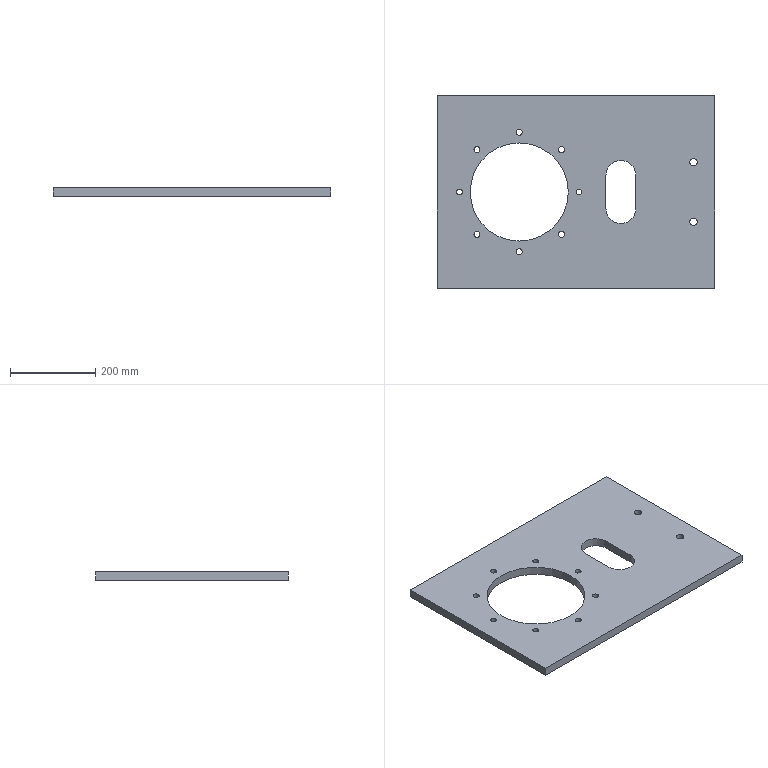Part | SolidWorks | features HoleWzd 3, CirPattern 2, FlatPattern 1, SMBaseFlange 1, SheetMetal 1 | 1 solid | 32 faces | box 650 x 450 x 20 mm | volume 4798629 mm3 | cylinder 24 | plane 8 | commonest cylinder face diameters 14 x16 17.5 x4 70 x2 230 x2
STEP:
#1=CARTESIAN_POINT('',(105.995,98.995,0.));
#2=VERTEX_POINT('',#1);
#3=CARTESIAN_POINT('',(91.995,98.995,0.));
#4=VERTEX_POINT('',#3);
#5=CARTESIAN_POINT('',(98.995,98.995,0.));
#6=DIRECTION('',(0.,0.,-1.));
#7=DIRECTION('',(-1.,0.,0.));
#8=AXIS2_PLACEMENT_3D('',#5,#6,#7);
#9=CIRCLE('',#8,7.);
#10=EDGE_CURVE('',#2,#4,#9,.T.);
#11=ORIENTED_EDGE('',*,*,#10,.F.);
#12=CARTESIAN_POINT('',(105.995,98.995,-20.));
#13=VERTEX_POINT('',#12);
#14=CARTESIAN_POINT('',(105.995,98.995,-20.));
#15=DIRECTION('',(0.,0.,-1.));
#16=VECTOR('',#15,1000.);
#17=LINE('',#14,#16);
#18=EDGE_CURVE('',#2,#13,#17,.T.);
#19=ORIENTED_EDGE('',*,*,#18,.T.);
#20=CARTESIAN_POINT('',(91.995,98.995,-20.));
#21=VERTEX_POINT('',#20);
#22=CARTESIAN_POINT('',(98.995,98.995,-20.));
#23=DIRECTION('',(0.,0.,-1.));
#24=DIRECTION('',(-1.,0.,0.));
#25=AXIS2_PLACEMENT_3D('',#22,#23,#24);
#26=CIRCLE('',#25,7.);
#27=EDGE_CURVE('',#13,#21,#26,.T.);
#28=ORIENTED_EDGE('',*,*,#27,.T.);
#29=CARTESIAN_POINT('',(91.995,98.995,-20.));
#30=DIRECTION('',(0.,0.,-1.));
#31=VECTOR('',#30,1000.);
#32=LINE('',#29,#31);
#33=EDGE_CURVE('',#4,#21,#32,.T.);
#34=ORIENTED_EDGE('',*,*,#33,.F.);
#35=EDGE_LOOP('',(#11,#19,#28,#34));
#36=FACE_OUTER_BOUND('',#35,.T.);
#37=CARTESIAN_POINT('',(98.995,98.995,-20.));
#38=DIRECTION('',(0.,0.,-1.));
#39=DIRECTION('',(-1.,0.,0.));
#40=AXIS2_PLACEMENT_3D('',#37,#38,#39);
#41=CYLINDRICAL_SURFACE('',#40,7.);
#42=ADVANCED_FACE('',(#36),#41,.F.);
#43=CARTESIAN_POINT('',(147.,0.,0.));
#44=VERTEX_POINT('',#43);
#45=CARTESIAN_POINT('',(133.,0.,0.));
#46=VERTEX_POINT('',#45);
#47=CARTESIAN_POINT('',(140.,0.,0.));
#48=DIRECTION('',(0.,0.,-1.));
#49=DIRECTION('',(-1.,0.,0.));
#50=AXIS2_PLACEMENT_3D('',#47,#48,#49);
#51=CIRCLE('',#50,7.);
#52=EDGE_CURVE('',#44,#46,#51,.T.);
#53=ORIENTED_EDGE('',*,*,#52,.F.);
#54=CARTESIAN_POINT('',(147.,0.,-20.));
#55=VERTEX_POINT('',#54);
#56=CARTESIAN_POINT('',(147.,0.,-20.));
#57=DIRECTION('',(0.,0.,-1.));
#58=VECTOR('',#57,1000.);
#59=LINE('',#56,#58);
#60=EDGE_CURVE('',#44,#55,#59,.T.);
#61=ORIENTED_EDGE('',*,*,#60,.T.);
#62=CARTESIAN_POINT('',(133.,0.,-20.));
#63=VERTEX_POINT('',#62);
#64=CARTESIAN_POINT('',(140.,0.,-20.));
#65=DIRECTION('',(0.,0.,-1.));
#66=DIRECTION('',(-1.,0.,0.));
#67=AXIS2_PLACEMENT_3D('',#64,#65,#66);
#68=CIRCLE('',#67,7.);
#69=EDGE_CURVE('',#55,#63,#68,.T.);
#70=ORIENTED_EDGE('',*,*,#69,.T.);
#71=CARTESIAN_POINT('',(133.,0.,-20.));
#72=DIRECTION('',(0.,0.,-1.));
#73=VECTOR('',#72,1000.);
#74=LINE('',#71,#73);
#75=EDGE_CURVE('',#46,#63,#74,.T.);
#76=ORIENTED_EDGE('',*,*,#75,.F.);
#77=EDGE_LOOP('',(#53,#61,#70,#76));
#78=FACE_OUTER_BOUND('',#77,.T.);
#79=CARTESIAN_POINT('',(140.,0.,-20.));
#80=DIRECTION('',(0.,0.,-1.));
#81=DIRECTION('',(-1.,0.,0.));
#82=AXIS2_PLACEMENT_3D('',#79,#80,#81);
#83=CYLINDRICAL_SURFACE('',#82,7.);
#84=ADVANCED_FACE('',(#78),#83,.F.);
#85=CARTESIAN_POINT('',(105.995,-98.995,0.));
#86=VERTEX_POINT('',#85);
#87=CARTESIAN_POINT('',(91.995,-98.995,0.));
#88=VERTEX_POINT('',#87);
#89=CARTESIAN_POINT('',(98.995,-98.995,0.));
#90=DIRECTION('',(0.,0.,-1.));
#91=DIRECTION('',(-1.,0.,0.));
#92=AXIS2_PLACEMENT_3D('',#89,#90,#91);
#93=CIRCLE('',#92,7.);
#94=EDGE_CURVE('',#86,#88,#93,.T.);
#95=ORIENTED_EDGE('',*,*,#94,.F.);
#96=CARTESIAN_POINT('',(105.995,-98.995,-20.));
#97=VERTEX_POINT('',#96);
#98=CARTESIAN_POINT('',(105.995,-98.995,-20.));
#99=DIRECTION('',(0.,0.,-1.));
#100=VECTOR('',#99,1000.);
#101=LINE('',#98,#100);
#102=EDGE_CURVE('',#86,#97,#101,.T.);
#103=ORIENTED_EDGE('',*,*,#102,.T.);
#104=CARTESIAN_POINT('',(91.995,-98.995,-20.));
#105=VERTEX_POINT('',#104);
#106=CARTESIAN_POINT('',(98.995,-98.995,-20.));
#107=DIRECTION('',(0.,0.,-1.));
#108=DIRECTION('',(-1.,0.,0.));
#109=AXIS2_PLACEMENT_3D('',#106,#107,#108);
#110=CIRCLE('',#109,7.);
#111=EDGE_CURVE('',#97,#105,#110,.T.);
#112=ORIENTED_EDGE('',*,*,#111,.T.);
#113=CARTESIAN_POINT('',(91.995,-98.995,-20.));
#114=DIRECTION('',(0.,0.,-1.));
#115=VECTOR('',#114,1000.);
#116=LINE('',#113,#115);
#117=EDGE_CURVE('',#88,#105,#116,.T.);
#118=ORIENTED_EDGE('',*,*,#117,.F.);
#119=EDGE_LOOP('',(#95,#103,#112,#118));
#120=FACE_OUTER_BOUND('',#119,.T.);
#121=CARTESIAN_POINT('',(98.995,-98.995,-20.));
#122=DIRECTION('',(0.,0.,-1.));
#123=DIRECTION('',(-1.,0.,0.));
#124=AXIS2_PLACEMENT_3D('',#121,#122,#123);
#125=CYLINDRICAL_SURFACE('',#124,7.);
#126=ADVANCED_FACE('',(#120),#125,.F.);
#127=CARTESIAN_POINT('',(7.,-140.,0.));
#128=VERTEX_POINT('',#127);
#129=CARTESIAN_POINT('',(-7.,-140.,0.));
#130=VERTEX_POINT('',#129);
#131=CARTESIAN_POINT('',(0.,-140.,0.));
#132=DIRECTION('',(0.,0.,-1.));
#133=DIRECTION('',(-1.,0.,0.));
#134=AXIS2_PLACEMENT_3D('',#131,#132,#133);
#135=CIRCLE('',#134,7.);
#136=EDGE_CURVE('',#128,#130,#135,.T.);
#137=ORIENTED_EDGE('',*,*,#136,.F.);
#138=CARTESIAN_POINT('',(7.,-140.,-20.));
#139=VERTEX_POINT('',#138);
#140=CARTESIAN_POINT('',(7.,-140.,-20.));
#141=DIRECTION('',(0.,0.,-1.));
#142=VECTOR('',#141,1000.);
#143=LINE('',#140,#142);
#144=EDGE_CURVE('',#128,#139,#143,.T.);
#145=ORIENTED_EDGE('',*,*,#144,.T.);
#146=CARTESIAN_POINT('',(-7.,-140.,-20.));
#147=VERTEX_POINT('',#146);
#148=CARTESIAN_POINT('',(0.,-140.,-20.));
#149=DIRECTION('',(0.,0.,-1.));
#150=DIRECTION('',(-1.,0.,0.));
#151=AXIS2_PLACEMENT_3D('',#148,#149,#150);
#152=CIRCLE('',#151,7.);
#153=EDGE_CURVE('',#139,#147,#152,.T.);
#154=ORIENTED_EDGE('',*,*,#153,.T.);
#155=CARTESIAN_POINT('',(-7.,-140.,-20.));
#156=DIRECTION('',(0.,0.,-1.));
#157=VECTOR('',#156,1000.);
#158=LINE('',#155,#157);
#159=EDGE_CURVE('',#130,#147,#158,.T.);
#160=ORIENTED_EDGE('',*,*,#159,.F.);
#161=EDGE_LOOP('',(#137,#145,#154,#160));
#162=FACE_OUTER_BOUND('',#161,.T.);
#163=CARTESIAN_POINT('',(0.,-140.,-20.));
#164=DIRECTION('',(0.,0.,-1.));
#165=DIRECTION('',(-1.,0.,0.));
#166=AXIS2_PLACEMENT_3D('',#163,#164,#165);
#167=CYLINDRICAL_SURFACE('',#166,7.);
#168=ADVANCED_FACE('',(#162),#167,.F.);
#169=CARTESIAN_POINT('',(-91.995,-98.995,0.));
#170=VERTEX_POINT('',#169);
#171=CARTESIAN_POINT('',(-105.995,-98.995,0.));
#172=VERTEX_POINT('',#171);
#173=CARTESIAN_POINT('',(-98.995,-98.995,0.));
#174=DIRECTION('',(0.,0.,-1.));
#175=DIRECTION('',(-1.,0.,0.));
#176=AXIS2_PLACEMENT_3D('',#173,#174,#175);
#177=CIRCLE('',#176,7.);
#178=EDGE_CURVE('',#170,#172,#177,.T.);
#179=ORIENTED_EDGE('',*,*,#178,.F.);
#180=CARTESIAN_POINT('',(-91.995,-98.995,-20.));
#181=VERTEX_POINT('',#180);
#182=CARTESIAN_POINT('',(-91.995,-98.995,-20.));
#183=DIRECTION('',(0.,0.,-1.));
#184=VECTOR('',#183,1000.);
#185=LINE('',#182,#184);
#186=EDGE_CURVE('',#170,#181,#185,.T.);
#187=ORIENTED_EDGE('',*,*,#186,.T.);
#188=CARTESIAN_POINT('',(-105.995,-98.995,-20.));
#189=VERTEX_POINT('',#188);
#190=CARTESIAN_POINT('',(-98.995,-98.995,-20.));
#191=DIRECTION('',(0.,0.,-1.));
#192=DIRECTION('',(-1.,0.,0.));
#193=AXIS2_PLACEMENT_3D('',#190,#191,#192);
#194=CIRCLE('',#193,7.);
#195=EDGE_CURVE('',#181,#189,#194,.T.);
#196=ORIENTED_EDGE('',*,*,#195,.T.);
#197=CARTESIAN_POINT('',(-105.995,-98.995,-20.));
#198=DIRECTION('',(0.,0.,-1.));
#199=VECTOR('',#198,1000.);
#200=LINE('',#197,#199);
#201=EDGE_CURVE('',#172,#189,#200,.T.);
#202=ORIENTED_EDGE('',*,*,#201,.F.);
#203=EDGE_LOOP('',(#179,#187,#196,#202));
#204=FACE_OUTER_BOUND('',#203,.T.);
#205=CARTESIAN_POINT('',(-98.995,-98.995,-20.));
#206=DIRECTION('',(0.,0.,-1.));
#207=DIRECTION('',(-1.,0.,0.));
#208=AXIS2_PLACEMENT_3D('',#205,#206,#207);
#209=CYLINDRICAL_SURFACE('',#208,7.);
#210=ADVANCED_FACE('',(#204),#209,.F.);
#211=CARTESIAN_POINT('',(-133.,0.,0.));
#212=VERTEX_POINT('',#211);
#213=CARTESIAN_POINT('',(-147.,0.,0.));
#214=VERTEX_POINT('',#213);
#215=CARTESIAN_POINT('',(-140.,0.,0.));
#216=DIRECTION('',(0.,0.,-1.));
#217=DIRECTION('',(-1.,0.,0.));
#218=AXIS2_PLACEMENT_3D('',#215,#216,#217);
#219=CIRCLE('',#218,7.);
#220=EDGE_CURVE('',#212,#214,#219,.T.);
#221=ORIENTED_EDGE('',*,*,#220,.F.);
#222=CARTESIAN_POINT('',(-133.,0.,-20.));
#223=VERTEX_POINT('',#222);
#224=CARTESIAN_POINT('',(-133.,0.,-20.));
#225=DIRECTION('',(0.,0.,-1.));
#226=VECTOR('',#225,1000.);
#227=LINE('',#224,#226);
#228=EDGE_CURVE('',#212,#223,#227,.T.);
#229=ORIENTED_EDGE('',*,*,#228,.T.);
#230=CARTESIAN_POINT('',(-147.,0.,-20.));
#231=VERTEX_POINT('',#230);
#232=CARTESIAN_POINT('',(-140.,0.,-20.));
#233=DIRECTION('',(0.,0.,-1.));
#234=DIRECTION('',(-1.,0.,0.));
#235=AXIS2_PLACEMENT_3D('',#232,#233,#234);
#236=CIRCLE('',#235,7.);
#237=EDGE_CURVE('',#223,#231,#236,.T.);
#238=ORIENTED_EDGE('',*,*,#237,.T.);
#239=CARTESIAN_POINT('',(-147.,0.,-20.));
#240=DIRECTION('',(0.,0.,-1.));
#241=VECTOR('',#240,1000.);
#242=LINE('',#239,#241);
#243=EDGE_CURVE('',#214,#231,#242,.T.);
#244=ORIENTED_EDGE('',*,*,#243,.F.);
#245=EDGE_LOOP('',(#221,#229,#238,#244));
#246=FACE_OUTER_BOUND('',#245,.T.);
#247=CARTESIAN_POINT('',(-140.,0.,-20.));
#248=DIRECTION('',(0.,0.,-1.));
#249=DIRECTION('',(-1.,0.,0.));
#250=AXIS2_PLACEMENT_3D('',#247,#248,#249);
#251=CYLINDRICAL_SURFACE('',#250,7.);
#252=ADVANCED_FACE('',(#246),#251,.F.);
#253=CARTESIAN_POINT('',(-91.995,98.995,0.));
#254=VERTEX_POINT('',#253);
#255=CARTESIAN_POINT('',(-105.995,98.995,0.));
#256=VERTEX_POINT('',#255);
#257=CARTESIAN_POINT('',(-98.995,98.995,0.));
#258=DIRECTION('',(0.,0.,-1.));
#259=DIRECTION('',(-1.,0.,0.));
#260=AXIS2_PLACEMENT_3D('',#257,#258,#259);
#261=CIRCLE('',#260,7.);
#262=EDGE_CURVE('',#254,#256,#261,.T.);
#263=ORIENTED_EDGE('',*,*,#262,.F.);
#264=CARTESIAN_POINT('',(-91.995,98.995,-20.));
#265=VERTEX_POINT('',#264);
#266=CARTESIAN_POINT('',(-91.995,98.995,-20.));
#267=DIRECTION('',(0.,0.,-1.));
#268=VECTOR('',#267,1000.);
#269=LINE('',#266,#268);
#270=EDGE_CURVE('',#254,#265,#269,.T.);
#271=ORIENTED_EDGE('',*,*,#270,.T.);
#272=CARTESIAN_POINT('',(-105.995,98.995,-20.));
#273=VERTEX_POINT('',#272);
#274=CARTESIAN_POINT('',(-98.995,98.995,-20.));
#275=DIRECTION('',(0.,0.,-1.));
#276=DIRECTION('',(-1.,0.,0.));
#277=AXIS2_PLACEMENT_3D('',#274,#275,#276);
#278=CIRCLE('',#277,7.);
#279=EDGE_CURVE('',#265,#273,#278,.T.);
#280=ORIENTED_EDGE('',*,*,#279,.T.);
#281=CARTESIAN_POINT('',(-105.995,98.995,-20.));
#282=DIRECTION('',(0.,0.,-1.));
#283=VECTOR('',#282,1000.);
#284=LINE('',#281,#283);
#285=EDGE_CURVE('',#256,#273,#284,.T.);
#286=ORIENTED_EDGE('',*,*,#285,.F.);
#287=EDGE_LOOP('',(#263,#271,#280,#286));
#288=FACE_OUTER_BOUND('',#287,.T.);
#289=CARTESIAN_POINT('',(-98.995,98.995,-20.));
#290=DIRECTION('',(0.,0.,-1.));
#291=DIRECTION('',(-1.,0.,0.));
#292=AXIS2_PLACEMENT_3D('',#289,#290,#291);
#293=CYLINDRICAL_SURFACE('',#292,7.);
#294=ADVANCED_FACE('',(#288),#293,.F.);
#295=CARTESIAN_POINT('',(7.,140.,0.));
#296=VERTEX_POINT('',#295);
#297=CARTESIAN_POINT('',(-7.,140.,0.));
#298=VERTEX_POINT('',#297);
#299=CARTESIAN_POINT('',(0.,140.,0.));
#300=DIRECTION('',(0.,0.,-1.));
#301=DIRECTION('',(-1.,0.,0.));
#302=AXIS2_PLACEMENT_3D('',#299,#300,#301);
#303=CIRCLE('',#302,7.);
#304=EDGE_CURVE('',#296,#298,#303,.T.);
#305=ORIENTED_EDGE('',*,*,#304,.F.);
#306=CARTESIAN_POINT('',(7.,140.,-20.));
#307=VERTEX_POINT('',#306);
#308=CARTESIAN_POINT('',(7.,140.,-20.));
#309=DIRECTION('',(0.,0.,-1.));
#310=VECTOR('',#309,1000.);
#311=LINE('',#308,#310);
#312=EDGE_CURVE('',#296,#307,#311,.T.);
#313=ORIENTED_EDGE('',*,*,#312,.T.);
#314=CARTESIAN_POINT('',(-7.,140.,-20.));
#315=VERTEX_POINT('',#314);
#316=CARTESIAN_POINT('',(0.,140.,-20.));
#317=DIRECTION('',(0.,0.,-1.));
#318=DIRECTION('',(-1.,0.,0.));
#319=AXIS2_PLACEMENT_3D('',#316,#317,#318);
#320=CIRCLE('',#319,7.);
#321=EDGE_CURVE('',#307,#315,#320,.T.);
#322=ORIENTED_EDGE('',*,*,#321,.T.);
#323=CARTESIAN_POINT('',(-7.,140.,-20.));
#324=DIRECTION('',(0.,0.,-1.));
#325=VECTOR('',#324,1000.);
#326=LINE('',#323,#325);
#327=EDGE_CURVE('',#298,#315,#326,.T.);
#328=ORIENTED_EDGE('',*,*,#327,.F.);
#329=EDGE_LOOP('',(#305,#313,#322,#328));
#330=FACE_OUTER_BOUND('',#329,.T.);
#331=CARTESIAN_POINT('',(0.,140.,-20.));
#332=DIRECTION('',(0.,0.,-1.));
#333=DIRECTION('',(-1.,0.,0.));
#334=AXIS2_PLACEMENT_3D('',#331,#332,#333);
#335=CYLINDRICAL_SURFACE('',#334,7.);
#336=ADVANCED_FACE('',(#330),#335,.F.);
#337=CARTESIAN_POINT('',(399.25,70.,-20.));
#338=VERTEX_POINT('',#337);
#339=CARTESIAN_POINT('',(416.75,70.,-20.));
#340=VERTEX_POINT('',#339);
#341=CARTESIAN_POINT('',(408.,70.,-20.));
#342=DIRECTION('',(0.,0.,1.));
#343=DIRECTION('',(1.,0.,0.));
#344=AXIS2_PLACEMENT_3D('',#341,#342,#343);
#345=CIRCLE('',#344,8.75);
#346=EDGE_CURVE('',#338,#340,#345,.T.);
#347=ORIENTED_EDGE('',*,*,#346,.F.);
#348=CARTESIAN_POINT('',(399.25,70.,0.));
#349=VERTEX_POINT('',#348);
#350=CARTESIAN_POINT('',(399.25,70.,0.));
#351=DIRECTION('',(0.,0.,1.));
#352=VECTOR('',#351,1000.);
#353=LINE('',#350,#352);
#354=EDGE_CURVE('',#338,#349,#353,.T.);
#355=ORIENTED_EDGE('',*,*,#354,.T.);
#356=CARTESIAN_POINT('',(416.75,70.,0.));
#357=VERTEX_POINT('',#356);
#358=CARTESIAN_POINT('',(408.,70.,0.));
#359=DIRECTION('',(0.,0.,1.));
#360=DIRECTION('',(1.,0.,0.));
#361=AXIS2_PLACEMENT_3D('',#358,#359,#360);
#362=CIRCLE('',#361,8.75);
#363=EDGE_CURVE('',#349,#357,#362,.T.);
#364=ORIENTED_EDGE('',*,*,#363,.T.);
#365=CARTESIAN_POINT('',(416.75,70.,0.));
#366=DIRECTION('',(0.,0.,1.));
#367=VECTOR('',#366,1000.);
#368=LINE('',#365,#367);
#369=EDGE_CURVE('',#340,#357,#368,.T.);
#370=ORIENTED_EDGE('',*,*,#369,.F.);
#371=EDGE_LOOP('',(#347,#355,#364,#370));
#372=FACE_OUTER_BOUND('',#371,.T.);
#373=CARTESIAN_POINT('',(408.,70.,0.));
#374=DIRECTION('',(0.,0.,1.));
#375=DIRECTION('',(1.,0.,0.));
#376=AXIS2_PLACEMENT_3D('',#373,#374,#375);
#377=CYLINDRICAL_SURFACE('',#376,8.75);
#378=ADVANCED_FACE('',(#372),#377,.F.);
#379=CARTESIAN_POINT('',(399.25,-70.,-20.));
#380=VERTEX_POINT('',#379);
#381=CARTESIAN_POINT('',(416.75,-70.,-20.));
#382=VERTEX_POINT('',#381);
#383=CARTESIAN_POINT('',(408.,-70.,-20.));
#384=DIRECTION('',(0.,0.,1.));
#385=DIRECTION('',(1.,0.,0.));
#386=AXIS2_PLACEMENT_3D('',#383,#384,#385);
#387=CIRCLE('',#386,8.75);
#388=EDGE_CURVE('',#380,#382,#387,.T.);
#389=ORIENTED_EDGE('',*,*,#388,.F.);
#390=CARTESIAN_POINT('',(399.25,-70.,0.));
#391=VERTEX_POINT('',#390);
#392=CARTESIAN_POINT('',(399.25,-70.,0.));
#393=DIRECTION('',(0.,0.,1.));
#394=VECTOR('',#393,1000.);
#395=LINE('',#392,#394);
#396=EDGE_CURVE('',#380,#391,#395,.T.);
#397=ORIENTED_EDGE('',*,*,#396,.T.);
#398=CARTESIAN_POINT('',(416.75,-70.,0.));
#399=VERTEX_POINT('',#398);
#400=CARTESIAN_POINT('',(408.,-70.,0.));
#401=DIRECTION('',(0.,0.,1.));
#402=DIRECTION('',(1.,0.,0.));
#403=AXIS2_PLACEMENT_3D('',#400,#401,#402);
#404=CIRCLE('',#403,8.75);
#405=EDGE_CURVE('',#391,#399,#404,.T.);
#406=ORIENTED_EDGE('',*,*,#405,.T.);
#407=CARTESIAN_POINT('',(416.75,-70.,0.));
#408=DIRECTION('',(0.,0.,1.));
#409=VECTOR('',#408,1000.);
#410=LINE('',#407,#409);
#411=EDGE_CURVE('',#382,#399,#410,.T.);
#412=ORIENTED_EDGE('',*,*,#411,.F.);
#413=EDGE_LOOP('',(#389,#397,#406,#412));
#414=FACE_OUTER_BOUND('',#413,.T.);
#415=CARTESIAN_POINT('',(408.,-70.,0.));
#416=DIRECTION('',(0.,0.,1.));
#417=DIRECTION('',(1.,0.,0.));
#418=AXIS2_PLACEMENT_3D('',#415,#416,#417);
#419=CYLINDRICAL_SURFACE('',#418,8.75);
#420=ADVANCED_FACE('',(#414),#419,.F.);
#421=CARTESIAN_POINT('',(-115.,0.,-20.));
#422=VERTEX_POINT('',#421);
#423=CARTESIAN_POINT('',(115.,0.,-20.));
#424=VERTEX_POINT('',#423);
#425=CARTESIAN_POINT('',(0.,0.,-20.));
#426=DIRECTION('',(0.,0.,1.));
#427=DIRECTION('',(1.,0.,0.));
#428=AXIS2_PLACEMENT_3D('',#425,#426,#427);
#429=CIRCLE('',#428,115.);
#430=EDGE_CURVE('',#422,#424,#429,.T.);
#431=ORIENTED_EDGE('',*,*,#430,.F.);
#432=CARTESIAN_POINT('',(-115.,0.,0.));
#433=VERTEX_POINT('',#432);
#434=CARTESIAN_POINT('',(-115.,0.,-20.));
#435=DIRECTION('',(0.,0.,1.));
#436=VECTOR('',#435,1000.);
#437=LINE('',#434,#436);
#438=EDGE_CURVE('',#422,#433,#437,.T.);
#439=ORIENTED_EDGE('',*,*,#438,.T.);
#440=CARTESIAN_POINT('',(115.,0.,0.));
#441=VERTEX_POINT('',#440);
#442=CARTESIAN_POINT('',(0.,0.,0.));
#443=DIRECTION('',(0.,0.,1.));
#444=DIRECTION('',(1.,0.,0.));
#445=AXIS2_PLACEMENT_3D('',#442,#443,#444);
#446=CIRCLE('',#445,115.);
#447=EDGE_CURVE('',#433,#441,#446,.T.);
#448=ORIENTED_EDGE('',*,*,#447,.T.);
#449=CARTESIAN_POINT('',(115.,0.,-20.));
#450=DIRECTION('',(0.,0.,1.));
#451=VECTOR('',#450,1000.);
#452=LINE('',#449,#451);
#453=EDGE_CURVE('',#424,#441,#452,.T.);
#454=ORIENTED_EDGE('',*,*,#453,.F.);
#455=EDGE_LOOP('',(#431,#439,#448,#454));
#456=FACE_OUTER_BOUND('',#455,.T.);
#457=CARTESIAN_POINT('',(0.,0.,-20.));
#458=DIRECTION('',(0.,0.,1.));
#459=DIRECTION('',(1.,0.,0.));
#460=AXIS2_PLACEMENT_3D('',#457,#458,#459);
#461=CYLINDRICAL_SURFACE('',#460,115.);
#462=ADVANCED_FACE('',(#456),#461,.F.);
#463=CARTESIAN_POINT('',(458.,-225.,0.));
#464=VERTEX_POINT('',#463);
#465=CARTESIAN_POINT('',(458.,225.,0.));
#466=VERTEX_POINT('',#465);
#467=CARTESIAN_POINT('',(458.,225.,0.));
#468=DIRECTION('',(0.,1.,0.));
#469=VECTOR('',#468,1000.);
#470=LINE('',#467,#469);
#471=EDGE_CURVE('',#464,#466,#470,.T.);
#472=ORIENTED_EDGE('',*,*,#471,.F.);
#473=CARTESIAN_POINT('',(458.,-225.,-20.));
#474=VERTEX_POINT('',#473);
#475=CARTESIAN_POINT('',(458.,-225.,-20.));
#476=DIRECTION('',(0.,0.,1.));
#477=VECTOR('',#476,1000.);
#478=LINE('',#475,#477);
#479=EDGE_CURVE('',#474,#464,#478,.T.);
#480=ORIENTED_EDGE('',*,*,#479,.F.);
#481=CARTESIAN_POINT('',(458.,225.,-20.));
#482=VERTEX_POINT('',#481);
#483=CARTESIAN_POINT('',(458.,225.,-20.));
#484=DIRECTION('',(0.,1.,0.));
#485=VECTOR('',#484,1000.);
#486=LINE('',#483,#485);
#487=EDGE_CURVE('',#474,#482,#486,.T.);
#488=ORIENTED_EDGE('',*,*,#487,.T.);
#489=CARTESIAN_POINT('',(458.,225.,-20.));
#490=DIRECTION('',(0.,0.,1.));
#491=VECTOR('',#490,1000.);
#492=LINE('',#489,#491);
#493=EDGE_CURVE('',#482,#466,#492,.T.);
#494=ORIENTED_EDGE('',*,*,#493,.T.);
#495=EDGE_LOOP('',(#472,#480,#488,#494));
#496=FACE_OUTER_BOUND('',#495,.T.);
#497=CARTESIAN_POINT('',(458.,225.,-20.));
#498=DIRECTION('',(1.,0.,0.));
#499=DIRECTION('',(0.,1.,0.));
#500=AXIS2_PLACEMENT_3D('',#497,#498,#499);
#501=PLANE('',#500);
#502=ADVANCED_FACE('',(#496),#501,.T.);
#503=CARTESIAN_POINT('',(-192.,-225.,0.));
#504=VERTEX_POINT('',#503);
#505=CARTESIAN_POINT('',(458.,-225.,0.));
#506=DIRECTION('',(1.,0.,0.));
#507=VECTOR('',#506,1000.);
#508=LINE('',#505,#507);
#509=EDGE_CURVE('',#504,#464,#508,.T.);
#510=ORIENTED_EDGE('',*,*,#509,.F.);
#511=CARTESIAN_POINT('',(-192.,-225.,-20.));
#512=VERTEX_POINT('',#511);
#513=CARTESIAN_POINT('',(-192.,-225.,-20.));
#514=DIRECTION('',(0.,0.,1.));
#515=VECTOR('',#514,1000.);
#516=LINE('',#513,#515);
#517=EDGE_CURVE('',#512,#504,#516,.T.);
#518=ORIENTED_EDGE('',*,*,#517,.F.);
#519=CARTESIAN_POINT('',(458.,-225.,-20.));
#520=DIRECTION('',(1.,0.,0.));
#521=VECTOR('',#520,1000.);
#522=LINE('',#519,#521);
#523=EDGE_CURVE('',#512,#474,#522,.T.);
#524=ORIENTED_EDGE('',*,*,#523,.T.);
#525=ORIENTED_EDGE('',*,*,#479,.T.);
#526=EDGE_LOOP('',(#510,#518,#524,#525));
#527=FACE_OUTER_BOUND('',#526,.T.);
#528=CARTESIAN_POINT('',(458.,-225.,-20.));
#529=DIRECTION('',(0.,-1.,0.));
#530=DIRECTION('',(1.,0.,0.));
#531=AXIS2_PLACEMENT_3D('',#528,#529,#530);
#532=PLANE('',#531);
#533=ADVANCED_FACE('',(#527),#532,.T.);
#534=CARTESIAN_POINT('',(-192.,225.,0.));
#535=VERTEX_POINT('',#534);
#536=CARTESIAN_POINT('',(-192.,225.,0.));
#537=DIRECTION('',(0.,-1.,0.));
#538=VECTOR('',#537,1000.);
#539=LINE('',#536,#538);
#540=EDGE_CURVE('',#535,#504,#539,.T.);
#541=ORIENTED_EDGE('',*,*,#540,.F.);
#542=CARTESIAN_POINT('',(-192.,225.,-20.));
#543=VERTEX_POINT('',#542);
#544=CARTESIAN_POINT('',(-192.,225.,-20.));
#545=DIRECTION('',(0.,0.,1.));
#546=VECTOR('',#545,1000.);
#547=LINE('',#544,#546);
#548=EDGE_CURVE('',#543,#535,#547,.T.);
#549=ORIENTED_EDGE('',*,*,#548,.F.);
#550=CARTESIAN_POINT('',(-192.,225.,-20.));
#551=DIRECTION('',(0.,-1.,0.));
#552=VECTOR('',#551,1000.);
#553=LINE('',#550,#552);
#554=EDGE_CURVE('',#543,#512,#553,.T.);
#555=ORIENTED_EDGE('',*,*,#554,.T.);
#556=ORIENTED_EDGE('',*,*,#517,.T.);
#557=EDGE_LOOP('',(#541,#549,#555,#556));
#558=FACE_OUTER_BOUND('',#557,.T.);
#559=CARTESIAN_POINT('',(-192.,225.,-20.));
#560=DIRECTION('',(-1.,0.,0.));
#561=DIRECTION('',(0.,-1.,0.));
#562=AXIS2_PLACEMENT_3D('',#559,#560,#561);
#563=PLANE('',#562);
#564=ADVANCED_FACE('',(#558),#563,.T.);
#565=CARTESIAN_POINT('',(458.,225.,0.));
#566=DIRECTION('',(-1.,0.,0.));
#567=VECTOR('',#566,1000.);
#568=LINE('',#565,#567);
#569=EDGE_CURVE('',#466,#535,#568,.T.);
#570=ORIENTED_EDGE('',*,*,#569,.F.);
#571=ORIENTED_EDGE('',*,*,#493,.F.);
#572=CARTESIAN_POINT('',(458.,225.,-20.));
#573=DIRECTION('',(-1.,0.,0.));
#574=VECTOR('',#573,1000.);
#575=LINE('',#572,#574);
#576=EDGE_CURVE('',#482,#543,#575,.T.);
#577=ORIENTED_EDGE('',*,*,#576,.T.);
#578=ORIENTED_EDGE('',*,*,#548,.T.);
#579=EDGE_LOOP('',(#570,#571,#577,#578));
#580=FACE_OUTER_BOUND('',#579,.T.);
#581=CARTESIAN_POINT('',(458.,225.,-20.));
#582=DIRECTION('',(0.,1.,0.));
#583=DIRECTION('',(-1.,0.,0.));
#584=AXIS2_PLACEMENT_3D('',#581,#582,#583);
#585=PLANE('',#584);
#586=ADVANCED_FACE('',(#580),#585,.T.);
#587=CARTESIAN_POINT('',(98.995,98.995,-20.));
#588=DIRECTION('',(0.,0.,-1.));
#589=DIRECTION('',(-1.,0.,0.));
#590=AXIS2_PLACEMENT_3D('',#587,#588,#589);
#591=CIRCLE('',#590,7.);
#592=EDGE_CURVE('',#21,#13,#591,.T.);
#593=ORIENTED_EDGE('',*,*,#592,.F.);
#594=ORIENTED_EDGE('',*,*,#27,.F.);
#595=EDGE_LOOP('',(#593,#594));
#596=FACE_BOUND('',#595,.T.);
#597=CARTESIAN_POINT('',(140.,0.,-20.));
#598=DIRECTION('',(0.,0.,-1.));
#599=DIRECTION('',(-1.,0.,0.));
#600=AXIS2_PLACEMENT_3D('',#597,#598,#599);
#601=CIRCLE('',#600,7.);
#602=EDGE_CURVE('',#63,#55,#601,.T.);
#603=ORIENTED_EDGE('',*,*,#602,.F.);
#604=ORIENTED_EDGE('',*,*,#69,.F.);
#605=EDGE_LOOP('',(#603,#604));
#606=FACE_BOUND('',#605,.T.);
#607=CARTESIAN_POINT('',(98.995,-98.995,-20.));
#608=DIRECTION('',(0.,0.,-1.));
#609=DIRECTION('',(-1.,0.,0.));
#610=AXIS2_PLACEMENT_3D('',#607,#608,#609);
#611=CIRCLE('',#610,7.);
#612=EDGE_CURVE('',#105,#97,#611,.T.);
#613=ORIENTED_EDGE('',*,*,#612,.F.);
#614=ORIENTED_EDGE('',*,*,#111,.F.);
#615=EDGE_LOOP('',(#613,#614));
#616=FACE_BOUND('',#615,.T.);
#617=CARTESIAN_POINT('',(0.,-140.,-20.));
#618=DIRECTION('',(0.,0.,-1.));
#619=DIRECTION('',(-1.,0.,0.));
#620=AXIS2_PLACEMENT_3D('',#617,#618,#619);
#621=CIRCLE('',#620,7.);
#622=EDGE_CURVE('',#147,#139,#621,.T.);
#623=ORIENTED_EDGE('',*,*,#622,.F.);
#624=ORIENTED_EDGE('',*,*,#153,.F.);
#625=EDGE_LOOP('',(#623,#624));
#626=FACE_BOUND('',#625,.T.);
#627=CARTESIAN_POINT('',(-98.995,-98.995,-20.));
#628=DIRECTION('',(0.,0.,-1.));
#629=DIRECTION('',(-1.,0.,0.));
#630=AXIS2_PLACEMENT_3D('',#627,#628,#629);
#631=CIRCLE('',#630,7.);
#632=EDGE_CURVE('',#189,#181,#631,.T.);
#633=ORIENTED_EDGE('',*,*,#632,.F.);
#634=ORIENTED_EDGE('',*,*,#195,.F.);
#635=EDGE_LOOP('',(#633,#634));
#636=FACE_BOUND('',#635,.T.);
#637=CARTESIAN_POINT('',(-140.,0.,-20.));
#638=DIRECTION('',(0.,0.,-1.));
#639=DIRECTION('',(-1.,0.,0.));
#640=AXIS2_PLACEMENT_3D('',#637,#638,#639);
#641=CIRCLE('',#640,7.);
#642=EDGE_CURVE('',#231,#223,#641,.T.);
#643=ORIENTED_EDGE('',*,*,#642,.F.);
#644=ORIENTED_EDGE('',*,*,#237,.F.);
#645=EDGE_LOOP('',(#643,#644));
#646=FACE_BOUND('',#645,.T.);
#647=CARTESIAN_POINT('',(-98.995,98.995,-20.));
#648=DIRECTION('',(0.,0.,-1.));
#649=DIRECTION('',(-1.,0.,0.));
#650=AXIS2_PLACEMENT_3D('',#647,#648,#649);
#651=CIRCLE('',#650,7.);
#652=EDGE_CURVE('',#273,#265,#651,.T.);
#653=ORIENTED_EDGE('',*,*,#652,.F.);
#654=ORIENTED_EDGE('',*,*,#279,.F.);
#655=EDGE_LOOP('',(#653,#654));
#656=FACE_BOUND('',#655,.T.);
#657=CARTESIAN_POINT('',(0.,140.,-20.));
#658=DIRECTION('',(0.,0.,-1.));
#659=DIRECTION('',(-1.,0.,0.));
#660=AXIS2_PLACEMENT_3D('',#657,#658,#659);
#661=CIRCLE('',#660,7.);
#662=EDGE_CURVE('',#315,#307,#661,.T.);
#663=ORIENTED_EDGE('',*,*,#662,.F.);
#664=ORIENTED_EDGE('',*,*,#321,.F.);
#665=EDGE_LOOP('',(#663,#664));
#666=FACE_BOUND('',#665,.T.);
#667=CARTESIAN_POINT('',(408.,70.,-20.));
#668=DIRECTION('',(0.,0.,1.));
#669=DIRECTION('',(1.,0.,0.));
#670=AXIS2_PLACEMENT_3D('',#667,#668,#669);
#671=CIRCLE('',#670,8.75);
#672=EDGE_CURVE('',#340,#338,#671,.T.);
#673=ORIENTED_EDGE('',*,*,#672,.T.);
#674=ORIENTED_EDGE('',*,*,#346,.T.);
#675=EDGE_LOOP('',(#673,#674));
#676=FACE_BOUND('',#675,.T.);
#677=CARTESIAN_POINT('',(408.,-70.,-20.));
#678=DIRECTION('',(0.,0.,1.));
#679=DIRECTION('',(1.,0.,0.));
#680=AXIS2_PLACEMENT_3D('',#677,#678,#679);
#681=CIRCLE('',#680,8.75);
#682=EDGE_CURVE('',#382,#380,#681,.T.);
#683=ORIENTED_EDGE('',*,*,#682,.T.);
#684=ORIENTED_EDGE('',*,*,#388,.T.);
#685=EDGE_LOOP('',(#683,#684));
#686=FACE_BOUND('',#685,.T.);
#687=CARTESIAN_POINT('',(273.,39.,-20.));
#688=VERTEX_POINT('',#687);
#689=CARTESIAN_POINT('',(203.,39.,-20.));
#690=VERTEX_POINT('',#689);
#691=CARTESIAN_POINT('',(238.,39.,-20.));
#692=DIRECTION('',(0.,0.,1.));
#693=DIRECTION('',(1.,0.,0.));
#694=AXIS2_PLACEMENT_3D('',#691,#692,#693);
#695=CIRCLE('',#694,35.);
#696=EDGE_CURVE('',#688,#690,#695,.T.);
#697=ORIENTED_EDGE('',*,*,#696,.T.);
#698=CARTESIAN_POINT('',(203.,-39.,-20.));
#699=VERTEX_POINT('',#698);
#700=CARTESIAN_POINT('',(203.,39.,-20.));
#701=DIRECTION('',(0.,-1.,0.));
#702=VECTOR('',#701,1000.);
#703=LINE('',#700,#702);
#704=EDGE_CURVE('',#690,#699,#703,.T.);
#705=ORIENTED_EDGE('',*,*,#704,.T.);
#706=CARTESIAN_POINT('',(273.,-39.,-20.));
#707=VERTEX_POINT('',#706);
#708=CARTESIAN_POINT('',(238.,-39.,-20.));
#709=DIRECTION('',(0.,0.,1.));
#710=DIRECTION('',(1.,0.,0.));
#711=AXIS2_PLACEMENT_3D('',#708,#709,#710);
#712=CIRCLE('',#711,35.);
#713=EDGE_CURVE('',#699,#707,#712,.T.);
#714=ORIENTED_EDGE('',*,*,#713,.T.);
#715=CARTESIAN_POINT('',(273.,39.,-20.));
#716=DIRECTION('',(0.,1.,0.));
#717=VECTOR('',#716,1000.);
#718=LINE('',#715,#717);
#719=EDGE_CURVE('',#707,#688,#718,.T.);
#720=ORIENTED_EDGE('',*,*,#719,.T.);
#721=EDGE_LOOP('',(#697,#705,#714,#720));
#722=FACE_BOUND('',#721,.T.);
#723=CARTESIAN_POINT('',(0.,0.,-20.));
#724=DIRECTION('',(0.,0.,1.));
#725=DIRECTION('',(1.,0.,0.));
#726=AXIS2_PLACEMENT_3D('',#723,#724,#725);
#727=CIRCLE('',#726,115.);
#728=EDGE_CURVE('',#424,#422,#727,.T.);
#729=ORIENTED_EDGE('',*,*,#728,.T.);
#730=ORIENTED_EDGE('',*,*,#430,.T.);
#731=EDGE_LOOP('',(#729,#730));
#732=FACE_BOUND('',#731,.T.);
#733=ORIENTED_EDGE('',*,*,#487,.F.);
#734=ORIENTED_EDGE('',*,*,#523,.F.);
#735=ORIENTED_EDGE('',*,*,#554,.F.);
#736=ORIENTED_EDGE('',*,*,#576,.F.);
#737=EDGE_LOOP('',(#733,#734,#735,#736));
#738=FACE_OUTER_BOUND('',#737,.T.);
#739=CARTESIAN_POINT('',(458.,-225.,-20.));
#740=DIRECTION('',(0.,0.,-1.));
#741=DIRECTION('',(-1.,0.,0.));
#742=AXIS2_PLACEMENT_3D('',#739,#740,#741);
#743=PLANE('',#742);
#744=ADVANCED_FACE('',(#596,#606,#616,#626,#636,#646,#656,#666,#676,#686,#722,#732,#738),#743,.T.);
#745=CARTESIAN_POINT('',(98.995,98.995,0.));
#746=DIRECTION('',(0.,0.,-1.));
#747=DIRECTION('',(-1.,0.,0.));
#748=AXIS2_PLACEMENT_3D('',#745,#746,#747);
#749=CIRCLE('',#748,7.);
#750=EDGE_CURVE('',#4,#2,#749,.T.);
#751=ORIENTED_EDGE('',*,*,#750,.T.);
#752=ORIENTED_EDGE('',*,*,#10,.T.);
#753=EDGE_LOOP('',(#751,#752));
#754=FACE_BOUND('',#753,.T.);
#755=CARTESIAN_POINT('',(140.,0.,0.));
#756=DIRECTION('',(0.,0.,-1.));
#757=DIRECTION('',(-1.,0.,0.));
#758=AXIS2_PLACEMENT_3D('',#755,#756,#757);
#759=CIRCLE('',#758,7.);
#760=EDGE_CURVE('',#46,#44,#759,.T.);
#761=ORIENTED_EDGE('',*,*,#760,.T.);
#762=ORIENTED_EDGE('',*,*,#52,.T.);
#763=EDGE_LOOP('',(#761,#762));
#764=FACE_BOUND('',#763,.T.);
#765=CARTESIAN_POINT('',(98.995,-98.995,0.));
#766=DIRECTION('',(0.,0.,-1.));
#767=DIRECTION('',(-1.,0.,0.));
#768=AXIS2_PLACEMENT_3D('',#765,#766,#767);
#769=CIRCLE('',#768,7.);
#770=EDGE_CURVE('',#88,#86,#769,.T.);
#771=ORIENTED_EDGE('',*,*,#770,.T.);
#772=ORIENTED_EDGE('',*,*,#94,.T.);
#773=EDGE_LOOP('',(#771,#772));
#774=FACE_BOUND('',#773,.T.);
#775=CARTESIAN_POINT('',(0.,-140.,0.));
#776=DIRECTION('',(0.,0.,-1.));
#777=DIRECTION('',(-1.,0.,0.));
#778=AXIS2_PLACEMENT_3D('',#775,#776,#777);
#779=CIRCLE('',#778,7.);
#780=EDGE_CURVE('',#130,#128,#779,.T.);
#781=ORIENTED_EDGE('',*,*,#780,.T.);
#782=ORIENTED_EDGE('',*,*,#136,.T.);
#783=EDGE_LOOP('',(#781,#782));
#784=FACE_BOUND('',#783,.T.);
#785=CARTESIAN_POINT('',(-98.995,-98.995,0.));
#786=DIRECTION('',(0.,0.,-1.));
#787=DIRECTION('',(-1.,0.,0.));
#788=AXIS2_PLACEMENT_3D('',#785,#786,#787);
#789=CIRCLE('',#788,7.);
#790=EDGE_CURVE('',#172,#170,#789,.T.);
#791=ORIENTED_EDGE('',*,*,#790,.T.);
#792=ORIENTED_EDGE('',*,*,#178,.T.);
#793=EDGE_LOOP('',(#791,#792));
#794=FACE_BOUND('',#793,.T.);
#795=CARTESIAN_POINT('',(-140.,0.,0.));
#796=DIRECTION('',(0.,0.,-1.));
#797=DIRECTION('',(-1.,0.,0.));
#798=AXIS2_PLACEMENT_3D('',#795,#796,#797);
#799=CIRCLE('',#798,7.);
#800=EDGE_CURVE('',#214,#212,#799,.T.);
#801=ORIENTED_EDGE('',*,*,#800,.T.);
#802=ORIENTED_EDGE('',*,*,#220,.T.);
#803=EDGE_LOOP('',(#801,#802));
#804=FACE_BOUND('',#803,.T.);
#805=CARTESIAN_POINT('',(-98.995,98.995,0.));
#806=DIRECTION('',(0.,0.,-1.));
#807=DIRECTION('',(-1.,0.,0.));
#808=AXIS2_PLACEMENT_3D('',#805,#806,#807);
#809=CIRCLE('',#808,7.);
#810=EDGE_CURVE('',#256,#254,#809,.T.);
#811=ORIENTED_EDGE('',*,*,#810,.T.);
#812=ORIENTED_EDGE('',*,*,#262,.T.);
#813=EDGE_LOOP('',(#811,#812));
#814=FACE_BOUND('',#813,.T.);
#815=CARTESIAN_POINT('',(0.,140.,0.));
#816=DIRECTION('',(0.,0.,-1.));
#817=DIRECTION('',(-1.,0.,0.));
#818=AXIS2_PLACEMENT_3D('',#815,#816,#817);
#819=CIRCLE('',#818,7.);
#820=EDGE_CURVE('',#298,#296,#819,.T.);
#821=ORIENTED_EDGE('',*,*,#820,.T.);
#822=ORIENTED_EDGE('',*,*,#304,.T.);
#823=EDGE_LOOP('',(#821,#822));
#824=FACE_BOUND('',#823,.T.);
#825=CARTESIAN_POINT('',(408.,70.,0.));
#826=DIRECTION('',(0.,0.,1.));
#827=DIRECTION('',(1.,0.,0.));
#828=AXIS2_PLACEMENT_3D('',#825,#826,#827);
#829=CIRCLE('',#828,8.75);
#830=EDGE_CURVE('',#357,#349,#829,.T.);
#831=ORIENTED_EDGE('',*,*,#830,.F.);
#832=ORIENTED_EDGE('',*,*,#363,.F.);
#833=EDGE_LOOP('',(#831,#832));
#834=FACE_BOUND('',#833,.T.);
#835=CARTESIAN_POINT('',(408.,-70.,0.));
#836=DIRECTION('',(0.,0.,1.));
#837=DIRECTION('',(1.,0.,0.));
#838=AXIS2_PLACEMENT_3D('',#835,#836,#837);
#839=CIRCLE('',#838,8.75);
#840=EDGE_CURVE('',#399,#391,#839,.T.);
#841=ORIENTED_EDGE('',*,*,#840,.F.);
#842=ORIENTED_EDGE('',*,*,#405,.F.);
#843=EDGE_LOOP('',(#841,#842));
#844=FACE_BOUND('',#843,.T.);
#845=CARTESIAN_POINT('',(203.,39.,0.));
#846=VERTEX_POINT('',#845);
#847=CARTESIAN_POINT('',(203.,-39.,0.));
#848=VERTEX_POINT('',#847);
#849=CARTESIAN_POINT('',(203.,39.,0.));
#850=DIRECTION('',(0.,-1.,0.));
#851=VECTOR('',#850,1000.);
#852=LINE('',#849,#851);
#853=EDGE_CURVE('',#846,#848,#852,.T.);
#854=ORIENTED_EDGE('',*,*,#853,.F.);
#855=CARTESIAN_POINT('',(273.,39.,0.));
#856=VERTEX_POINT('',#855);
#857=CARTESIAN_POINT('',(238.,39.,0.));
#858=DIRECTION('',(0.,0.,1.));
#859=DIRECTION('',(1.,0.,0.));
#860=AXIS2_PLACEMENT_3D('',#857,#858,#859);
#861=CIRCLE('',#860,35.);
#862=EDGE_CURVE('',#856,#846,#861,.T.);
#863=ORIENTED_EDGE('',*,*,#862,.F.);
#864=CARTESIAN_POINT('',(273.,-39.,0.));
#865=VERTEX_POINT('',#864);
#866=CARTESIAN_POINT('',(273.,39.,0.));
#867=DIRECTION('',(0.,1.,0.));
#868=VECTOR('',#867,1000.);
#869=LINE('',#866,#868);
#870=EDGE_CURVE('',#865,#856,#869,.T.);
#871=ORIENTED_EDGE('',*,*,#870,.F.);
#872=CARTESIAN_POINT('',(238.,-39.,0.));
#873=DIRECTION('',(0.,0.,1.));
#874=DIRECTION('',(1.,0.,0.));
#875=AXIS2_PLACEMENT_3D('',#872,#873,#874);
#876=CIRCLE('',#875,35.);
#877=EDGE_CURVE('',#848,#865,#876,.T.);
#878=ORIENTED_EDGE('',*,*,#877,.F.);
#879=EDGE_LOOP('',(#854,#863,#871,#878));
#880=FACE_BOUND('',#879,.T.);
#881=CARTESIAN_POINT('',(0.,0.,0.));
#882=DIRECTION('',(0.,0.,1.));
#883=DIRECTION('',(1.,0.,0.));
#884=AXIS2_PLACEMENT_3D('',#881,#882,#883);
#885=CIRCLE('',#884,115.);
#886=EDGE_CURVE('',#441,#433,#885,.T.);
#887=ORIENTED_EDGE('',*,*,#886,.F.);
#888=ORIENTED_EDGE('',*,*,#447,.F.);
#889=EDGE_LOOP('',(#887,#888));
#890=FACE_BOUND('',#889,.T.);
#891=ORIENTED_EDGE('',*,*,#471,.T.);
#892=ORIENTED_EDGE('',*,*,#569,.T.);
#893=ORIENTED_EDGE('',*,*,#540,.T.);
#894=ORIENTED_EDGE('',*,*,#509,.T.);
#895=EDGE_LOOP('',(#891,#892,#893,#894));
#896=FACE_OUTER_BOUND('',#895,.T.);
#897=CARTESIAN_POINT('',(458.,-225.,0.));
#898=DIRECTION('',(0.,0.,-1.));
#899=DIRECTION('',(-1.,0.,0.));
#900=AXIS2_PLACEMENT_3D('',#897,#898,#899);
#901=PLANE('',#900);
#902=ADVANCED_FACE('',(#754,#764,#774,#784,#794,#804,#814,#824,#834,#844,#880,#890,#896),#901,.F.);
#903=ORIENTED_EDGE('',*,*,#438,.F.);
#904=ORIENTED_EDGE('',*,*,#728,.F.);
#905=ORIENTED_EDGE('',*,*,#453,.T.);
#906=ORIENTED_EDGE('',*,*,#886,.T.);
#907=EDGE_LOOP('',(#903,#904,#905,#906));
#908=FACE_OUTER_BOUND('',#907,.T.);
#909=CARTESIAN_POINT('',(0.,0.,-20.));
#910=DIRECTION('',(0.,0.,1.));
#911=DIRECTION('',(1.,0.,0.));
#912=AXIS2_PLACEMENT_3D('',#909,#910,#911);
#913=CYLINDRICAL_SURFACE('',#912,115.);
#914=ADVANCED_FACE('',(#908),#913,.F.);
#915=ORIENTED_EDGE('',*,*,#862,.T.);
#916=CARTESIAN_POINT('',(203.,39.,-20.));
#917=DIRECTION('',(0.,0.,1.));
#918=VECTOR('',#917,1000.);
#919=LINE('',#916,#918);
#920=EDGE_CURVE('',#690,#846,#919,.T.);
#921=ORIENTED_EDGE('',*,*,#920,.F.);
#922=ORIENTED_EDGE('',*,*,#696,.F.);
#923=CARTESIAN_POINT('',(273.,39.,-20.));
#924=DIRECTION('',(0.,0.,1.));
#925=VECTOR('',#924,1000.);
#926=LINE('',#923,#925);
#927=EDGE_CURVE('',#688,#856,#926,.T.);
#928=ORIENTED_EDGE('',*,*,#927,.T.);
#929=EDGE_LOOP('',(#915,#921,#922,#928));
#930=FACE_OUTER_BOUND('',#929,.T.);
#931=CARTESIAN_POINT('',(238.,39.,-20.));
#932=DIRECTION('',(0.,0.,1.));
#933=DIRECTION('',(1.,0.,0.));
#934=AXIS2_PLACEMENT_3D('',#931,#932,#933);
#935=CYLINDRICAL_SURFACE('',#934,35.);
#936=ADVANCED_FACE('',(#930),#935,.F.);
#937=ORIENTED_EDGE('',*,*,#870,.T.);
#938=ORIENTED_EDGE('',*,*,#927,.F.);
#939=ORIENTED_EDGE('',*,*,#719,.F.);
#940=CARTESIAN_POINT('',(273.,-39.,-20.));
#941=DIRECTION('',(0.,0.,1.));
#942=VECTOR('',#941,1000.);
#943=LINE('',#940,#942);
#944=EDGE_CURVE('',#707,#865,#943,.T.);
#945=ORIENTED_EDGE('',*,*,#944,.T.);
#946=EDGE_LOOP('',(#937,#938,#939,#945));
#947=FACE_OUTER_BOUND('',#946,.T.);
#948=CARTESIAN_POINT('',(273.,39.,-20.));
#949=DIRECTION('',(1.,0.,0.));
#950=DIRECTION('',(0.,0.,-1.));
#951=AXIS2_PLACEMENT_3D('',#948,#949,#950);
#952=PLANE('',#951);
#953=ADVANCED_FACE('',(#947),#952,.F.);
#954=ORIENTED_EDGE('',*,*,#877,.T.);
#955=ORIENTED_EDGE('',*,*,#944,.F.);
#956=ORIENTED_EDGE('',*,*,#713,.F.);
#957=CARTESIAN_POINT('',(203.,-39.,-20.));
#958=DIRECTION('',(0.,0.,1.));
#959=VECTOR('',#958,1000.);
#960=LINE('',#957,#959);
#961=EDGE_CURVE('',#699,#848,#960,.T.);
#962=ORIENTED_EDGE('',*,*,#961,.T.);
#963=EDGE_LOOP('',(#954,#955,#956,#962));
#964=FACE_OUTER_BOUND('',#963,.T.);
#965=CARTESIAN_POINT('',(238.,-39.,-20.));
#966=DIRECTION('',(0.,0.,1.));
#967=DIRECTION('',(1.,0.,0.));
#968=AXIS2_PLACEMENT_3D('',#965,#966,#967);
#969=CYLINDRICAL_SURFACE('',#968,35.);
#970=ADVANCED_FACE('',(#964),#969,.F.);
#971=ORIENTED_EDGE('',*,*,#853,.T.);
#972=ORIENTED_EDGE('',*,*,#961,.F.);
#973=ORIENTED_EDGE('',*,*,#704,.F.);
#974=ORIENTED_EDGE('',*,*,#920,.T.);
#975=EDGE_LOOP('',(#971,#972,#973,#974));
#976=FACE_OUTER_BOUND('',#975,.T.);
#977=CARTESIAN_POINT('',(203.,39.,-20.));
#978=DIRECTION('',(-1.,0.,0.));
#979=DIRECTION('',(0.,0.,1.));
#980=AXIS2_PLACEMENT_3D('',#977,#978,#979);
#981=PLANE('',#980);
#982=ADVANCED_FACE('',(#976),#981,.F.);
#983=ORIENTED_EDGE('',*,*,#396,.F.);
#984=ORIENTED_EDGE('',*,*,#682,.F.);
#985=ORIENTED_EDGE('',*,*,#411,.T.);
#986=ORIENTED_EDGE('',*,*,#840,.T.);
#987=EDGE_LOOP('',(#983,#984,#985,#986));
#988=FACE_OUTER_BOUND('',#987,.T.);
#989=CARTESIAN_POINT('',(408.,-70.,0.));
#990=DIRECTION('',(0.,0.,1.));
#991=DIRECTION('',(1.,0.,0.));
#992=AXIS2_PLACEMENT_3D('',#989,#990,#991);
#993=CYLINDRICAL_SURFACE('',#992,8.75);
#994=ADVANCED_FACE('',(#988),#993,.F.);
#995=ORIENTED_EDGE('',*,*,#354,.F.);
#996=ORIENTED_EDGE('',*,*,#672,.F.);
#997=ORIENTED_EDGE('',*,*,#369,.T.);
#998=ORIENTED_EDGE('',*,*,#830,.T.);
#999=EDGE_LOOP('',(#995,#996,#997,#998));
#1000=FACE_OUTER_BOUND('',#999,.T.);
#1001=CARTESIAN_POINT('',(408.,70.,0.));
#1002=DIRECTION('',(0.,0.,1.));
#1003=DIRECTION('',(1.,0.,0.));
#1004=AXIS2_PLACEMENT_3D('',#1001,#1002,#1003);
#1005=CYLINDRICAL_SURFACE('',#1004,8.75);
#1006=ADVANCED_FACE('',(#1000),#1005,.F.);
#1007=ORIENTED_EDGE('',*,*,#312,.F.);
#1008=ORIENTED_EDGE('',*,*,#820,.F.);
#1009=ORIENTED_EDGE('',*,*,#327,.T.);
#1010=ORIENTED_EDGE('',*,*,#662,.T.);
#1011=EDGE_LOOP('',(#1007,#1008,#1009,#1010));
#1012=FACE_OUTER_BOUND('',#1011,.T.);
#1013=CARTESIAN_POINT('',(0.,140.,-20.));
#1014=DIRECTION('',(0.,0.,-1.));
#1015=DIRECTION('',(-1.,0.,0.));
#1016=AXIS2_PLACEMENT_3D('',#1013,#1014,#1015);
#1017=CYLINDRICAL_SURFACE('',#1016,7.);
#1018=ADVANCED_FACE('',(#1012),#1017,.F.);
#1019=ORIENTED_EDGE('',*,*,#270,.F.);
#1020=ORIENTED_EDGE('',*,*,#810,.F.);
#1021=ORIENTED_EDGE('',*,*,#285,.T.);
#1022=ORIENTED_EDGE('',*,*,#652,.T.);
#1023=EDGE_LOOP('',(#1019,#1020,#1021,#1022));
#1024=FACE_OUTER_BOUND('',#1023,.T.);
#1025=CARTESIAN_POINT('',(-98.995,98.995,-20.));
#1026=DIRECTION('',(0.,0.,-1.));
#1027=DIRECTION('',(-1.,0.,0.));
#1028=AXIS2_PLACEMENT_3D('',#1025,#1026,#1027);
#1029=CYLINDRICAL_SURFACE('',#1028,7.);
#1030=ADVANCED_FACE('',(#1024),#1029,.F.);
#1031=ORIENTED_EDGE('',*,*,#228,.F.);
#1032=ORIENTED_EDGE('',*,*,#800,.F.);
#1033=ORIENTED_EDGE('',*,*,#243,.T.);
#1034=ORIENTED_EDGE('',*,*,#642,.T.);
#1035=EDGE_LOOP('',(#1031,#1032,#1033,#1034));
#1036=FACE_OUTER_BOUND('',#1035,.T.);
#1037=CARTESIAN_POINT('',(-140.,0.,-20.));
#1038=DIRECTION('',(0.,0.,-1.));
#1039=DIRECTION('',(-1.,0.,0.));
#1040=AXIS2_PLACEMENT_3D('',#1037,#1038,#1039);
#1041=CYLINDRICAL_SURFACE('',#1040,7.);
#1042=ADVANCED_FACE('',(#1036),#1041,.F.);
#1043=ORIENTED_EDGE('',*,*,#186,.F.);
#1044=ORIENTED_EDGE('',*,*,#790,.F.);
#1045=ORIENTED_EDGE('',*,*,#201,.T.);
#1046=ORIENTED_EDGE('',*,*,#632,.T.);
#1047=EDGE_LOOP('',(#1043,#1044,#1045,#1046));
#1048=FACE_OUTER_BOUND('',#1047,.T.);
#1049=CARTESIAN_POINT('',(-98.995,-98.995,-20.));
#1050=DIRECTION('',(0.,0.,-1.));
#1051=DIRECTION('',(-1.,0.,0.));
#1052=AXIS2_PLACEMENT_3D('',#1049,#1050,#1051);
#1053=CYLINDRICAL_SURFACE('',#1052,7.);
#1054=ADVANCED_FACE('',(#1048),#1053,.F.);
#1055=ORIENTED_EDGE('',*,*,#144,.F.);
#1056=ORIENTED_EDGE('',*,*,#780,.F.);
#1057=ORIENTED_EDGE('',*,*,#159,.T.);
#1058=ORIENTED_EDGE('',*,*,#622,.T.);
#1059=EDGE_LOOP('',(#1055,#1056,#1057,#1058));
#1060=FACE_OUTER_BOUND('',#1059,.T.);
#1061=CARTESIAN_POINT('',(0.,-140.,-20.));
#1062=DIRECTION('',(0.,0.,-1.));
#1063=DIRECTION('',(-1.,0.,0.));
#1064=AXIS2_PLACEMENT_3D('',#1061,#1062,#1063);
#1065=CYLINDRICAL_SURFACE('',#1064,7.);
#1066=ADVANCED_FACE('',(#1060),#1065,.F.);
#1067=ORIENTED_EDGE('',*,*,#102,.F.);
#1068=ORIENTED_EDGE('',*,*,#770,.F.);
#1069=ORIENTED_EDGE('',*,*,#117,.T.);
#1070=ORIENTED_EDGE('',*,*,#612,.T.);
#1071=EDGE_LOOP('',(#1067,#1068,#1069,#1070));
#1072=FACE_OUTER_BOUND('',#1071,.T.);
#1073=CARTESIAN_POINT('',(98.995,-98.995,-20.));
#1074=DIRECTION('',(0.,0.,-1.));
#1075=DIRECTION('',(-1.,0.,0.));
#1076=AXIS2_PLACEMENT_3D('',#1073,#1074,#1075);
#1077=CYLINDRICAL_SURFACE('',#1076,7.);
#1078=ADVANCED_FACE('',(#1072),#1077,.F.);
#1079=ORIENTED_EDGE('',*,*,#60,.F.);
#1080=ORIENTED_EDGE('',*,*,#760,.F.);
#1081=ORIENTED_EDGE('',*,*,#75,.T.);
#1082=ORIENTED_EDGE('',*,*,#602,.T.);
#1083=EDGE_LOOP('',(#1079,#1080,#1081,#1082));
#1084=FACE_OUTER_BOUND('',#1083,.T.);
#1085=CARTESIAN_POINT('',(140.,0.,-20.));
#1086=DIRECTION('',(0.,0.,-1.));
#1087=DIRECTION('',(-1.,0.,0.));
#1088=AXIS2_PLACEMENT_3D('',#1085,#1086,#1087);
#1089=CYLINDRICAL_SURFACE('',#1088,7.);
#1090=ADVANCED_FACE('',(#1084),#1089,.F.);
#1091=ORIENTED_EDGE('',*,*,#18,.F.);
#1092=ORIENTED_EDGE('',*,*,#750,.F.);
#1093=ORIENTED_EDGE('',*,*,#33,.T.);
#1094=ORIENTED_EDGE('',*,*,#592,.T.);
#1095=EDGE_LOOP('',(#1091,#1092,#1093,#1094));
#1096=FACE_OUTER_BOUND('',#1095,.T.);
#1097=CARTESIAN_POINT('',(98.995,98.995,-20.));
#1098=DIRECTION('',(0.,0.,-1.));
#1099=DIRECTION('',(-1.,0.,0.));
#1100=AXIS2_PLACEMENT_3D('',#1097,#1098,#1099);
#1101=CYLINDRICAL_SURFACE('',#1100,7.);
#1102=ADVANCED_FACE('',(#1096),#1101,.F.);
#1103=CLOSED_SHELL('',(#42,#84,#126,#168,#210,#252,#294,#336,#378,#420,#462,#502,#533,#564,#586,#744,#902,#914,#936,#953,#970,#982,#994,#1006,#1018,#1030,#1042,#1054,#1066,#1078,#1090,#1102));
#1104=MANIFOLD_SOLID_BREP('',#1103);
#1105=CARTESIAN_POINT('',(0.,0.,0.));
#1106=DIRECTION('',(0.,0.,1.));
#1107=DIRECTION('',(1.,0.,0.));
#1108=AXIS2_PLACEMENT_3D('',#1105,#1106,#1107);
#1109=(LENGTH_UNIT()NAMED_UNIT(*)SI_UNIT(.MILLI.,.METRE.));
#1110=UNCERTAINTY_MEASURE_WITH_UNIT(LENGTH_MEASURE(0.00001),#1109,'','');
#1111=(NAMED_UNIT(*)PLANE_ANGLE_UNIT()SI_UNIT($,.RADIAN.));
#1112=(NAMED_UNIT(*)SI_UNIT($,.STERADIAN.)SOLID_ANGLE_UNIT());
#1113=(GEOMETRIC_REPRESENTATION_CONTEXT(3)GLOBAL_UNCERTAINTY_ASSIGNED_CONTEXT((#1110))GLOBAL_UNIT_ASSIGNED_CONTEXT((#1109,#1111,#1112))REPRESENTATION_CONTEXT('',''));
#1114=ADVANCED_BREP_SHAPE_REPRESENTATION('',(#1104,#1108),#1113);